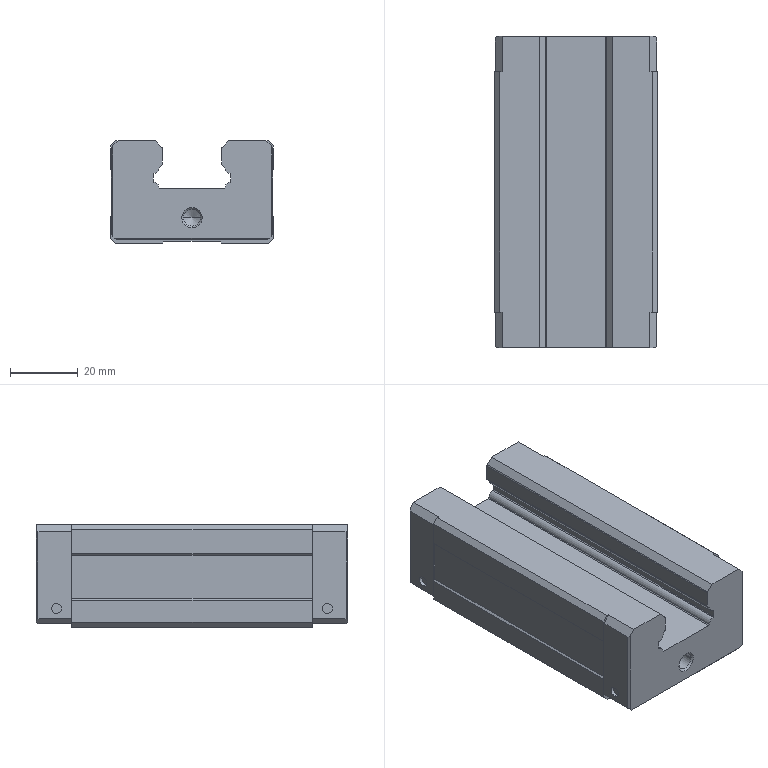Part | 1 solid | 126 faces | box 48 x 92 x 30.2 mm | volume 103686 mm3 | plane 66 | cylinder 36 | cone 24 | commonest cylinder face diameters 4.917 x12 3 x8 0.6 x4 0.594 x2 0.985 x2 0.988 x2